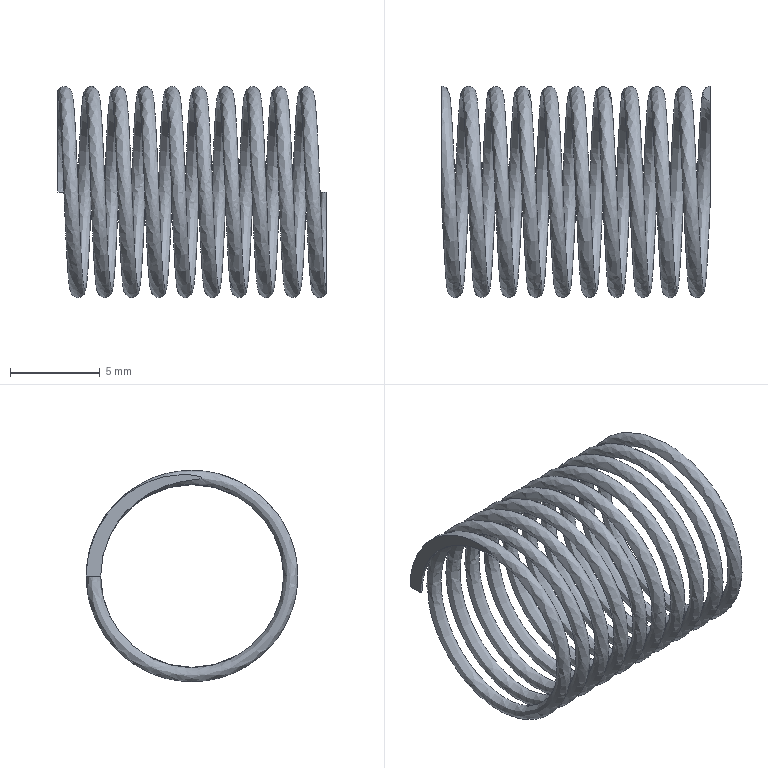Part | NX | features BREP 1, DATUM_CSYS 1 | 1 solid | 5 faces | box 15 x 11.8 x 11.8 mm | volume 171.601 mm3 | plane 4 | spline 1
STEP:
#1=CARTESIAN_POINT('',(76.,5.1,8.));
#2=VERTEX_POINT('',#1);
#3=CARTESIAN_POINT('',(76.,5.9,8.));
#4=VERTEX_POINT('',#3);
#5=CARTESIAN_POINT('',(76.,5.5,8.));
#6=DIRECTION('',(0.,0.,-1.));
#7=DIRECTION('',(0.,-1.,0.));
#8=AXIS2_PLACEMENT_3D('',#5,#6,#7);
#9=CIRCLE('',#8,0.4);
#10=EDGE_CURVE('',#2,#4,#9,.T.);
#11=ORIENTED_EDGE('',*,*,#10,.F.);
#12=CARTESIAN_POINT('',(76.,5.9,8.));
#13=DIRECTION('',(0.,-1.,0.));
#14=VECTOR('',#13,1000.);
#15=LINE('',#12,#14);
#16=EDGE_CURVE('',#4,#2,#15,.T.);
#17=ORIENTED_EDGE('',*,*,#16,.F.);
#18=EDGE_LOOP('',(#11,#17));
#19=FACE_BOUND('',#18,.T.);
#20=CARTESIAN_POINT('',(75.8,5.5,8.));
#21=DIRECTION('',(0.,0.,1.));
#22=DIRECTION('',(0.,-1.,0.));
#23=AXIS2_PLACEMENT_3D('',#20,#21,#22);
#24=PLANE('',#23);
#25=ADVANCED_FACE('',(#19),#24,.T.);
#26=CARTESIAN_POINT('',(76.,-0.5373,2.526));
#27=VERTEX_POINT('',#26);
#28=CARTESIAN_POINT('',(61.4,5.5,8.));
#29=VERTEX_POINT('',#28);
#30=CARTESIAN_POINT('',(76.,-0.5373,2.526));
#31=CARTESIAN_POINT('',(75.843,-3.895,2.856));
#32=CARTESIAN_POINT('',(75.761,-5.5,5.447));
#33=CARTESIAN_POINT('',(75.65,-5.5,8.));
#34=CARTESIAN_POINT('',(75.173,-5.5,19.));
#35=CARTESIAN_POINT('',(75.377,5.5,19.));
#36=CARTESIAN_POINT('',(74.9,5.5,8.));
#37=CARTESIAN_POINT('',(74.423,5.5,-3.));
#38=CARTESIAN_POINT('',(74.627,-5.5,-3.));
#39=CARTESIAN_POINT('',(74.15,-5.5,8.));
#40=CARTESIAN_POINT('',(73.673,-5.5,19.));
#41=CARTESIAN_POINT('',(73.877,5.5,19.));
#42=CARTESIAN_POINT('',(73.4,5.5,8.));
#43=CARTESIAN_POINT('',(72.923,5.5,-3.));
#44=CARTESIAN_POINT('',(73.127,-5.5,-3.));
#45=CARTESIAN_POINT('',(72.65,-5.5,8.));
#46=CARTESIAN_POINT('',(72.173,-5.5,19.));
#47=CARTESIAN_POINT('',(72.377,5.5,19.));
#48=CARTESIAN_POINT('',(71.9,5.5,8.));
#49=CARTESIAN_POINT('',(71.423,5.5,-3.));
#50=CARTESIAN_POINT('',(71.627,-5.5,-3.));
#51=CARTESIAN_POINT('',(71.15,-5.5,8.));
#52=CARTESIAN_POINT('',(70.673,-5.5,19.));
#53=CARTESIAN_POINT('',(70.877,5.5,19.));
#54=CARTESIAN_POINT('',(70.4,5.5,8.));
#55=CARTESIAN_POINT('',(69.923,5.5,-3.));
#56=CARTESIAN_POINT('',(70.127,-5.5,-3.));
#57=CARTESIAN_POINT('',(69.65,-5.5,8.));
#58=CARTESIAN_POINT('',(69.173,-5.5,19.));
#59=CARTESIAN_POINT('',(69.377,5.5,19.));
#60=CARTESIAN_POINT('',(68.9,5.5,8.));
#61=CARTESIAN_POINT('',(68.423,5.5,-3.));
#62=CARTESIAN_POINT('',(68.627,-5.5,-3.));
#63=CARTESIAN_POINT('',(68.15,-5.5,8.));
#64=CARTESIAN_POINT('',(67.673,-5.5,19.));
#65=CARTESIAN_POINT('',(67.877,5.5,19.));
#66=CARTESIAN_POINT('',(67.4,5.5,8.));
#67=CARTESIAN_POINT('',(66.923,5.5,-3.));
#68=CARTESIAN_POINT('',(67.127,-5.5,-3.));
#69=CARTESIAN_POINT('',(66.65,-5.5,8.));
#70=CARTESIAN_POINT('',(66.173,-5.5,19.));
#71=CARTESIAN_POINT('',(66.377,5.5,19.));
#72=CARTESIAN_POINT('',(65.9,5.5,8.));
#73=CARTESIAN_POINT('',(65.423,5.5,-3.));
#74=CARTESIAN_POINT('',(65.627,-5.5,-3.));
#75=CARTESIAN_POINT('',(65.15,-5.5,8.));
#76=CARTESIAN_POINT('',(64.673,-5.5,19.));
#77=CARTESIAN_POINT('',(64.877,5.5,19.));
#78=CARTESIAN_POINT('',(64.4,5.5,8.));
#79=CARTESIAN_POINT('',(63.923,5.5,-3.));
#80=CARTESIAN_POINT('',(64.127,-5.5,-3.));
#81=CARTESIAN_POINT('',(63.65,-5.5,8.));
#82=CARTESIAN_POINT('',(63.173,-5.5,19.));
#83=CARTESIAN_POINT('',(63.377,5.5,19.));
#84=CARTESIAN_POINT('',(62.9,5.5,8.));
#85=CARTESIAN_POINT('',(62.423,5.5,-3.));
#86=CARTESIAN_POINT('',(62.627,-5.5,-3.));
#87=CARTESIAN_POINT('',(62.15,-5.5,8.));
#88=CARTESIAN_POINT('',(61.673,-5.5,19.));
#89=CARTESIAN_POINT('',(61.877,5.5,19.));
#90=CARTESIAN_POINT('',(61.4,5.5,8.));
#91=(BOUNDED_CURVE()B_SPLINE_CURVE(3,(#30,#31,#32,#33,#34,#35,#36,#37,#38,#39,#40,#41,#42,#43,#44,#45,#46,#47,#48,#49,#50,#51,#52,#53,#54,#55,#56,#57,#58,#59,#60,#61,#62,#63,#64,#65,#66,#67,#68,#69,#70,#71,#72,#73,#74,#75,#76,#77,#78,#79,#80,#81,#82,#83,#84,#85,#86,#87,#88,#89,#90),.UNSPECIFIED.,.F.,.F.)B_SPLINE_CURVE_WITH_KNOTS((4,3,3,3,3,3,3,3,3,3,3,3,3,3,3,3,3,3,3,3,4),(0.,0.02442,0.07576,0.1271,0.1785,0.2298,0.2811,0.3325,0.3838,0.4352,0.4865,0.5379,0.5892,0.6406,0.6919,0.7433,0.7946,0.846,0.8973,0.9487,1.),.PIECEWISE_BEZIER_KNOTS.)CURVE()GEOMETRIC_REPRESENTATION_ITEM()RATIONAL_B_SPLINE_CURVE((0.5012,0.5167,0.683,1.,0.3333,0.3333,1.,0.3333,0.3333,1.,0.3333,0.3333,1.,0.3333,0.3333,1.,0.3333,0.3333,1.,0.3333,0.3333,1.,0.3333,0.3333,1.,0.3333,0.3333,1.,0.3333,0.3333,1.,0.3333,0.3333,1.,0.3333,0.3333,1.,0.3333,0.3333,1.,0.3333,0.3333,1.,0.3333,0.3333,1.,0.3333,0.3333,1.,0.3333,0.3333,1.,0.3333,0.3333,1.,0.3333,0.3333,1.,0.3333,0.3333,1.))REPRESENTATION_ITEM(''));
#92=EDGE_CURVE('',#27,#29,#91,.T.);
#93=ORIENTED_EDGE('',*,*,#92,.F.);
#94=CARTESIAN_POINT('',(76.,5.1,8.));
#95=CARTESIAN_POINT('',(76.,5.1,7.271));
#96=CARTESIAN_POINT('',(76.,4.87,6.189));
#97=CARTESIAN_POINT('',(76.,4.149,4.925));
#98=CARTESIAN_POINT('',(76.,3.427,4.106));
#99=CARTESIAN_POINT('',(76.,2.563,3.453));
#100=CARTESIAN_POINT('',(76.,1.74,3.054));
#101=CARTESIAN_POINT('',(76.,1.056,2.834));
#102=CARTESIAN_POINT('',(76.,0.5256,2.714));
#103=CARTESIAN_POINT('',(76.,0.08176,2.645));
#104=CARTESIAN_POINT('',(76.,-0.2455,2.613));
#105=CARTESIAN_POINT('',(76.,-0.4071,2.578));
#106=CARTESIAN_POINT('',(76.,-0.5328,2.572));
#107=CARTESIAN_POINT('',(76.,-0.5373,2.526));
#108=B_SPLINE_CURVE_WITH_KNOTS('',3,(#94,#95,#96,#97,#98,#99,#100,#101,#102,#103,#104,#105,#106,#107),.UNSPECIFIED.,.F.,.F.,(4,1,1,1,1,1,1,1,1,1,1,4),(0.,0.002182,0.003272,0.004363,0.005454,0.006545,0.00709,0.007636,0.008181,0.008454,0.00859,0.008726),.UNSPECIFIED.);
#109=EDGE_CURVE('',#2,#27,#108,.T.);
#110=ORIENTED_EDGE('',*,*,#109,.F.);
#111=ORIENTED_EDGE('',*,*,#10,.T.);
#112=CARTESIAN_POINT('',(76.,-0.5373,2.526));
#113=CARTESIAN_POINT('',(76.,-0.5425,2.474));
#114=CARTESIAN_POINT('',(76.,-0.3977,2.446));
#115=CARTESIAN_POINT('',(76.,-0.2237,2.388));
#116=CARTESIAN_POINT('',(76.,0.04228,2.353));
#117=CARTESIAN_POINT('',(76.,0.3421,2.331));
#118=CARTESIAN_POINT('',(76.,0.7489,2.333));
#119=CARTESIAN_POINT('',(76.,1.259,2.386));
#120=CARTESIAN_POINT('',(76.,2.047,2.563));
#121=CARTESIAN_POINT('',(76.,2.993,2.956));
#122=CARTESIAN_POINT('',(76.,3.989,3.658));
#123=CARTESIAN_POINT('',(76.,4.817,4.562));
#124=CARTESIAN_POINT('',(76.,5.639,5.973));
#125=CARTESIAN_POINT('',(76.,5.9,7.182));
#126=CARTESIAN_POINT('',(76.,5.9,8.));
#127=B_SPLINE_CURVE_WITH_KNOTS('',3,(#112,#113,#114,#115,#116,#117,#118,#119,#120,#121,#122,#123,#124,#125,#126),.UNSPECIFIED.,.F.,.F.,(4,1,1,1,1,1,1,1,1,1,1,1,4),(0.,0.0001559,0.0003119,0.0006238,0.0009356,0.001248,0.001871,0.002495,0.003743,0.00499,0.006238,0.007485,0.00998),.UNSPECIFIED.);
#128=EDGE_CURVE('',#27,#4,#127,.T.);
#129=ORIENTED_EDGE('',*,*,#128,.F.);
#130=ORIENTED_EDGE('',*,*,#92,.T.);
#131=CARTESIAN_POINT('',(61.,5.9,8.));
#132=VERTEX_POINT('',#131);
#133=CARTESIAN_POINT('',(61.,5.9,8.));
#134=CARTESIAN_POINT('',(61.4,5.9,8.));
#135=CARTESIAN_POINT('',(61.4,5.5,8.));
#136=(BOUNDED_CURVE()B_SPLINE_CURVE(2,(#133,#134,#135),.UNSPECIFIED.,.F.,.F.)B_SPLINE_CURVE_WITH_KNOTS((3,3),(0.,1.),.PIECEWISE_BEZIER_KNOTS.)CURVE()GEOMETRIC_REPRESENTATION_ITEM()RATIONAL_B_SPLINE_CURVE((0.8038,0.634,1.))REPRESENTATION_ITEM(''));
#137=EDGE_CURVE('',#132,#29,#136,.T.);
#138=ORIENTED_EDGE('',*,*,#137,.F.);
#139=CARTESIAN_POINT('',(61.,5.1,8.));
#140=VERTEX_POINT('',#139);
#141=CARTESIAN_POINT('',(61.,5.1,8.));
#142=CARTESIAN_POINT('',(61.,5.1,8.783));
#143=CARTESIAN_POINT('',(61.,4.747,10.331));
#144=CARTESIAN_POINT('',(61.,3.515,11.895));
#145=CARTESIAN_POINT('',(61.,2.218,12.748));
#146=CARTESIAN_POINT('',(61.,1.309,13.105));
#147=CARTESIAN_POINT('',(61.,0.5535,13.282));
#148=CARTESIAN_POINT('',(61.,0.07717,13.354));
#149=CARTESIAN_POINT('',(61.,-0.2742,13.393));
#150=CARTESIAN_POINT('',(61.,-0.4254,13.421));
#151=CARTESIAN_POINT('',(61.,-0.5471,13.447));
#152=CARTESIAN_POINT('',(61.,-0.4994,13.543));
#153=CARTESIAN_POINT('',(61.,-0.3702,13.564));
#154=CARTESIAN_POINT('',(61.,-0.1891,13.617));
#155=CARTESIAN_POINT('',(61.,0.145,13.66));
#156=CARTESIAN_POINT('',(61.,0.6237,13.677));
#157=CARTESIAN_POINT('',(61.,1.379,13.606));
#158=CARTESIAN_POINT('',(61.,2.307,13.358));
#159=CARTESIAN_POINT('',(61.,3.323,12.839));
#160=CARTESIAN_POINT('',(61.,4.517,11.882));
#161=CARTESIAN_POINT('',(61.,5.594,10.279));
#162=CARTESIAN_POINT('',(61.,5.9,8.766));
#163=CARTESIAN_POINT('',(61.,5.9,8.));
#164=B_SPLINE_CURVE_WITH_KNOTS('',3,(#141,#142,#143,#144,#145,#146,#147,#148,#149,#150,#151,#152,#153,#154,#155,#156,#157,#158,#159,#160,#161,#162,#163),.UNSPECIFIED.,.F.,.F.,(4,1,1,1,1,1,1,1,1,1,1,1,1,1,1,1,1,1,1,1,4),(0.,0.002341,0.004682,0.005852,0.007022,0.007608,0.008193,0.008485,0.008632,0.008705,0.008778,0.008924,0.00907,0.009363,0.009948,0.01053,0.0117,0.01287,0.01404,0.01639,0.01873),.UNSPECIFIED.);
#165=EDGE_CURVE('',#140,#132,#164,.T.);
#166=ORIENTED_EDGE('',*,*,#165,.F.);
#167=CARTESIAN_POINT('',(61.4,5.5,8.));
#168=CARTESIAN_POINT('',(61.4,5.1,8.));
#169=CARTESIAN_POINT('',(61.,5.1,8.));
#170=(BOUNDED_CURVE()B_SPLINE_CURVE(2,(#167,#168,#169),.UNSPECIFIED.,.F.,.F.)B_SPLINE_CURVE_WITH_KNOTS((3,3),(0.,1.),.PIECEWISE_BEZIER_KNOTS.)CURVE()GEOMETRIC_REPRESENTATION_ITEM()RATIONAL_B_SPLINE_CURVE((1.,0.634,0.8038))REPRESENTATION_ITEM(''));
#171=EDGE_CURVE('',#29,#140,#170,.T.);
#172=ORIENTED_EDGE('',*,*,#171,.F.);
#173=EDGE_LOOP('',(#93,#110,#111,#129,#130,#138,#166,#172));
#174=FACE_BOUND('',#173,.T.);
#175=CARTESIAN_POINT('',(76.4,5.5,8.));
#176=CARTESIAN_POINT('',(75.923,5.5,-3.));
#177=CARTESIAN_POINT('',(76.127,-5.5,-3.));
#178=CARTESIAN_POINT('',(75.65,-5.5,8.));
#179=CARTESIAN_POINT('',(75.173,-5.5,19.));
#180=CARTESIAN_POINT('',(75.377,5.5,19.));
#181=CARTESIAN_POINT('',(74.9,5.5,8.));
#182=CARTESIAN_POINT('',(74.423,5.5,-3.));
#183=CARTESIAN_POINT('',(74.627,-5.5,-3.));
#184=CARTESIAN_POINT('',(74.15,-5.5,8.));
#185=CARTESIAN_POINT('',(73.673,-5.5,19.));
#186=CARTESIAN_POINT('',(73.877,5.5,19.));
#187=CARTESIAN_POINT('',(73.4,5.5,8.));
#188=CARTESIAN_POINT('',(72.923,5.5,-3.));
#189=CARTESIAN_POINT('',(73.127,-5.5,-3.));
#190=CARTESIAN_POINT('',(72.65,-5.5,8.));
#191=CARTESIAN_POINT('',(72.173,-5.5,19.));
#192=CARTESIAN_POINT('',(72.377,5.5,19.));
#193=CARTESIAN_POINT('',(71.9,5.5,8.));
#194=CARTESIAN_POINT('',(71.423,5.5,-3.));
#195=CARTESIAN_POINT('',(71.627,-5.5,-3.));
#196=CARTESIAN_POINT('',(71.15,-5.5,8.));
#197=CARTESIAN_POINT('',(70.673,-5.5,19.));
#198=CARTESIAN_POINT('',(70.877,5.5,19.));
#199=CARTESIAN_POINT('',(70.4,5.5,8.));
#200=CARTESIAN_POINT('',(69.923,5.5,-3.));
#201=CARTESIAN_POINT('',(70.127,-5.5,-3.));
#202=CARTESIAN_POINT('',(69.65,-5.5,8.));
#203=CARTESIAN_POINT('',(69.173,-5.5,19.));
#204=CARTESIAN_POINT('',(69.377,5.5,19.));
#205=CARTESIAN_POINT('',(68.9,5.5,8.));
#206=CARTESIAN_POINT('',(68.423,5.5,-3.));
#207=CARTESIAN_POINT('',(68.627,-5.5,-3.));
#208=CARTESIAN_POINT('',(68.15,-5.5,8.));
#209=CARTESIAN_POINT('',(67.673,-5.5,19.));
#210=CARTESIAN_POINT('',(67.877,5.5,19.));
#211=CARTESIAN_POINT('',(67.4,5.5,8.));
#212=CARTESIAN_POINT('',(66.923,5.5,-3.));
#213=CARTESIAN_POINT('',(67.127,-5.5,-3.));
#214=CARTESIAN_POINT('',(66.65,-5.5,8.));
#215=CARTESIAN_POINT('',(66.173,-5.5,19.));
#216=CARTESIAN_POINT('',(66.377,5.5,19.));
#217=CARTESIAN_POINT('',(65.9,5.5,8.));
#218=CARTESIAN_POINT('',(65.423,5.5,-3.));
#219=CARTESIAN_POINT('',(65.627,-5.5,-3.));
#220=CARTESIAN_POINT('',(65.15,-5.5,8.));
#221=CARTESIAN_POINT('',(64.673,-5.5,19.));
#222=CARTESIAN_POINT('',(64.877,5.5,19.));
#223=CARTESIAN_POINT('',(64.4,5.5,8.));
#224=CARTESIAN_POINT('',(63.923,5.5,-3.));
#225=CARTESIAN_POINT('',(64.127,-5.5,-3.));
#226=CARTESIAN_POINT('',(63.65,-5.5,8.));
#227=CARTESIAN_POINT('',(63.173,-5.5,19.));
#228=CARTESIAN_POINT('',(63.377,5.5,19.));
#229=CARTESIAN_POINT('',(62.9,5.5,8.));
#230=CARTESIAN_POINT('',(62.423,5.5,-3.));
#231=CARTESIAN_POINT('',(62.627,-5.5,-3.));
#232=CARTESIAN_POINT('',(62.15,-5.5,8.));
#233=CARTESIAN_POINT('',(61.673,-5.5,19.));
#234=CARTESIAN_POINT('',(61.877,5.5,19.));
#235=CARTESIAN_POINT('',(61.4,5.5,8.));
#236=CARTESIAN_POINT('',(76.4,4.807,8.));
#237=CARTESIAN_POINT('',(75.923,4.807,-1.614));
#238=CARTESIAN_POINT('',(76.127,-4.807,-1.614));
#239=CARTESIAN_POINT('',(75.65,-4.807,8.));
#240=CARTESIAN_POINT('',(75.173,-4.807,17.614));
#241=CARTESIAN_POINT('',(75.377,4.807,17.614));
#242=CARTESIAN_POINT('',(74.9,4.807,8.));
#243=CARTESIAN_POINT('',(74.423,4.807,-1.614));
#244=CARTESIAN_POINT('',(74.627,-4.807,-1.614));
#245=CARTESIAN_POINT('',(74.15,-4.807,8.));
#246=CARTESIAN_POINT('',(73.673,-4.807,17.614));
#247=CARTESIAN_POINT('',(73.877,4.807,17.614));
#248=CARTESIAN_POINT('',(73.4,4.807,8.));
#249=CARTESIAN_POINT('',(72.923,4.807,-1.614));
#250=CARTESIAN_POINT('',(73.127,-4.807,-1.614));
#251=CARTESIAN_POINT('',(72.65,-4.807,8.));
#252=CARTESIAN_POINT('',(72.173,-4.807,17.614));
#253=CARTESIAN_POINT('',(72.377,4.807,17.614));
#254=CARTESIAN_POINT('',(71.9,4.807,8.));
#255=CARTESIAN_POINT('',(71.423,4.807,-1.614));
#256=CARTESIAN_POINT('',(71.627,-4.807,-1.614));
#257=CARTESIAN_POINT('',(71.15,-4.807,8.));
#258=CARTESIAN_POINT('',(70.673,-4.807,17.614));
#259=CARTESIAN_POINT('',(70.877,4.807,17.614));
#260=CARTESIAN_POINT('',(70.4,4.807,8.));
#261=CARTESIAN_POINT('',(69.923,4.807,-1.614));
#262=CARTESIAN_POINT('',(70.127,-4.807,-1.614));
#263=CARTESIAN_POINT('',(69.65,-4.807,8.));
#264=CARTESIAN_POINT('',(69.173,-4.807,17.614));
#265=CARTESIAN_POINT('',(69.377,4.807,17.614));
#266=CARTESIAN_POINT('',(68.9,4.807,8.));
#267=CARTESIAN_POINT('',(68.423,4.807,-1.614));
#268=CARTESIAN_POINT('',(68.627,-4.807,-1.614));
#269=CARTESIAN_POINT('',(68.15,-4.807,8.));
#270=CARTESIAN_POINT('',(67.673,-4.807,17.614));
#271=CARTESIAN_POINT('',(67.877,4.807,17.614));
#272=CARTESIAN_POINT('',(67.4,4.807,8.));
#273=CARTESIAN_POINT('',(66.923,4.807,-1.614));
#274=CARTESIAN_POINT('',(67.127,-4.807,-1.614));
#275=CARTESIAN_POINT('',(66.65,-4.807,8.));
#276=CARTESIAN_POINT('',(66.173,-4.807,17.614));
#277=CARTESIAN_POINT('',(66.377,4.807,17.614));
#278=CARTESIAN_POINT('',(65.9,4.807,8.));
#279=CARTESIAN_POINT('',(65.423,4.807,-1.614));
#280=CARTESIAN_POINT('',(65.627,-4.807,-1.614));
#281=CARTESIAN_POINT('',(65.15,-4.807,8.));
#282=CARTESIAN_POINT('',(64.673,-4.807,17.614));
#283=CARTESIAN_POINT('',(64.877,4.807,17.614));
#284=CARTESIAN_POINT('',(64.4,4.807,8.));
#285=CARTESIAN_POINT('',(63.923,4.807,-1.614));
#286=CARTESIAN_POINT('',(64.127,-4.807,-1.614));
#287=CARTESIAN_POINT('',(63.65,-4.807,8.));
#288=CARTESIAN_POINT('',(63.173,-4.807,17.614));
#289=CARTESIAN_POINT('',(63.377,4.807,17.614));
#290=CARTESIAN_POINT('',(62.9,4.807,8.));
#291=CARTESIAN_POINT('',(62.423,4.807,-1.614));
#292=CARTESIAN_POINT('',(62.627,-4.807,-1.614));
#293=CARTESIAN_POINT('',(62.15,-4.807,8.));
#294=CARTESIAN_POINT('',(61.673,-4.807,17.614));
#295=CARTESIAN_POINT('',(61.877,4.807,17.614));
#296=CARTESIAN_POINT('',(61.4,4.807,8.));
#297=CARTESIAN_POINT('',(75.8,5.154,8.));
#298=CARTESIAN_POINT('',(75.323,5.154,-2.307));
#299=CARTESIAN_POINT('',(75.527,-5.154,-2.307));
#300=CARTESIAN_POINT('',(75.05,-5.154,8.));
#301=CARTESIAN_POINT('',(74.573,-5.154,18.307));
#302=CARTESIAN_POINT('',(74.777,5.154,18.307));
#303=CARTESIAN_POINT('',(74.3,5.154,8.));
#304=CARTESIAN_POINT('',(73.823,5.154,-2.307));
#305=CARTESIAN_POINT('',(74.027,-5.154,-2.307));
#306=CARTESIAN_POINT('',(73.55,-5.154,8.));
#307=CARTESIAN_POINT('',(73.073,-5.154,18.307));
#308=CARTESIAN_POINT('',(73.277,5.154,18.307));
#309=CARTESIAN_POINT('',(72.8,5.154,8.));
#310=CARTESIAN_POINT('',(72.323,5.154,-2.307));
#311=CARTESIAN_POINT('',(72.527,-5.154,-2.307));
#312=CARTESIAN_POINT('',(72.05,-5.154,8.));
#313=CARTESIAN_POINT('',(71.573,-5.154,18.307));
#314=CARTESIAN_POINT('',(71.777,5.154,18.307));
#315=CARTESIAN_POINT('',(71.3,5.154,8.));
#316=CARTESIAN_POINT('',(70.823,5.154,-2.307));
#317=CARTESIAN_POINT('',(71.027,-5.154,-2.307));
#318=CARTESIAN_POINT('',(70.55,-5.154,8.));
#319=CARTESIAN_POINT('',(70.073,-5.154,18.307));
#320=CARTESIAN_POINT('',(70.277,5.154,18.307));
#321=CARTESIAN_POINT('',(69.8,5.154,8.));
#322=CARTESIAN_POINT('',(69.323,5.154,-2.307));
#323=CARTESIAN_POINT('',(69.527,-5.154,-2.307));
#324=CARTESIAN_POINT('',(69.05,-5.154,8.));
#325=CARTESIAN_POINT('',(68.573,-5.154,18.307));
#326=CARTESIAN_POINT('',(68.777,5.154,18.307));
#327=CARTESIAN_POINT('',(68.3,5.154,8.));
#328=CARTESIAN_POINT('',(67.823,5.154,-2.307));
#329=CARTESIAN_POINT('',(68.027,-5.154,-2.307));
#330=CARTESIAN_POINT('',(67.55,-5.154,8.));
#331=CARTESIAN_POINT('',(67.073,-5.154,18.307));
#332=CARTESIAN_POINT('',(67.277,5.154,18.307));
#333=CARTESIAN_POINT('',(66.8,5.154,8.));
#334=CARTESIAN_POINT('',(66.323,5.154,-2.307));
#335=CARTESIAN_POINT('',(66.527,-5.154,-2.307));
#336=CARTESIAN_POINT('',(66.05,-5.154,8.));
#337=CARTESIAN_POINT('',(65.573,-5.154,18.307));
#338=CARTESIAN_POINT('',(65.777,5.154,18.307));
#339=CARTESIAN_POINT('',(65.3,5.154,8.));
#340=CARTESIAN_POINT('',(64.823,5.154,-2.307));
#341=CARTESIAN_POINT('',(65.027,-5.154,-2.307));
#342=CARTESIAN_POINT('',(64.55,-5.154,8.));
#343=CARTESIAN_POINT('',(64.073,-5.154,18.307));
#344=CARTESIAN_POINT('',(64.277,5.154,18.307));
#345=CARTESIAN_POINT('',(63.8,5.154,8.));
#346=CARTESIAN_POINT('',(63.323,5.154,-2.307));
#347=CARTESIAN_POINT('',(63.527,-5.154,-2.307));
#348=CARTESIAN_POINT('',(63.05,-5.154,8.));
#349=CARTESIAN_POINT('',(62.573,-5.154,18.307));
#350=CARTESIAN_POINT('',(62.777,5.154,18.307));
#351=CARTESIAN_POINT('',(62.3,5.154,8.));
#352=CARTESIAN_POINT('',(61.823,5.154,-2.307));
#353=CARTESIAN_POINT('',(62.027,-5.154,-2.307));
#354=CARTESIAN_POINT('',(61.55,-5.154,8.));
#355=CARTESIAN_POINT('',(61.073,-5.154,18.307));
#356=CARTESIAN_POINT('',(61.277,5.154,18.307));
#357=CARTESIAN_POINT('',(60.8,5.154,8.));
#358=CARTESIAN_POINT('',(75.2,5.5,8.));
#359=CARTESIAN_POINT('',(74.723,5.5,-3.));
#360=CARTESIAN_POINT('',(74.927,-5.5,-3.));
#361=CARTESIAN_POINT('',(74.45,-5.5,8.));
#362=CARTESIAN_POINT('',(73.973,-5.5,19.));
#363=CARTESIAN_POINT('',(74.177,5.5,19.));
#364=CARTESIAN_POINT('',(73.7,5.5,8.));
#365=CARTESIAN_POINT('',(73.223,5.5,-3.));
#366=CARTESIAN_POINT('',(73.427,-5.5,-3.));
#367=CARTESIAN_POINT('',(72.95,-5.5,8.));
#368=CARTESIAN_POINT('',(72.473,-5.5,19.));
#369=CARTESIAN_POINT('',(72.677,5.5,19.));
#370=CARTESIAN_POINT('',(72.2,5.5,8.));
#371=CARTESIAN_POINT('',(71.723,5.5,-3.));
#372=CARTESIAN_POINT('',(71.927,-5.5,-3.));
#373=CARTESIAN_POINT('',(71.45,-5.5,8.));
#374=CARTESIAN_POINT('',(70.973,-5.5,19.));
#375=CARTESIAN_POINT('',(71.177,5.5,19.));
#376=CARTESIAN_POINT('',(70.7,5.5,8.));
#377=CARTESIAN_POINT('',(70.223,5.5,-3.));
#378=CARTESIAN_POINT('',(70.427,-5.5,-3.));
#379=CARTESIAN_POINT('',(69.95,-5.5,8.));
#380=CARTESIAN_POINT('',(69.473,-5.5,19.));
#381=CARTESIAN_POINT('',(69.677,5.5,19.));
#382=CARTESIAN_POINT('',(69.2,5.5,8.));
#383=CARTESIAN_POINT('',(68.723,5.5,-3.));
#384=CARTESIAN_POINT('',(68.927,-5.5,-3.));
#385=CARTESIAN_POINT('',(68.45,-5.5,8.));
#386=CARTESIAN_POINT('',(67.973,-5.5,19.));
#387=CARTESIAN_POINT('',(68.177,5.5,19.));
#388=CARTESIAN_POINT('',(67.7,5.5,8.));
#389=CARTESIAN_POINT('',(67.223,5.5,-3.));
#390=CARTESIAN_POINT('',(67.427,-5.5,-3.));
#391=CARTESIAN_POINT('',(66.95,-5.5,8.));
#392=CARTESIAN_POINT('',(66.473,-5.5,19.));
#393=CARTESIAN_POINT('',(66.677,5.5,19.));
#394=CARTESIAN_POINT('',(66.2,5.5,8.));
#395=CARTESIAN_POINT('',(65.723,5.5,-3.));
#396=CARTESIAN_POINT('',(65.927,-5.5,-3.));
#397=CARTESIAN_POINT('',(65.45,-5.5,8.));
#398=CARTESIAN_POINT('',(64.973,-5.5,19.));
#399=CARTESIAN_POINT('',(65.177,5.5,19.));
#400=CARTESIAN_POINT('',(64.7,5.5,8.));
#401=CARTESIAN_POINT('',(64.223,5.5,-3.));
#402=CARTESIAN_POINT('',(64.427,-5.5,-3.));
#403=CARTESIAN_POINT('',(63.95,-5.5,8.));
#404=CARTESIAN_POINT('',(63.473,-5.5,19.));
#405=CARTESIAN_POINT('',(63.677,5.5,19.));
#406=CARTESIAN_POINT('',(63.2,5.5,8.));
#407=CARTESIAN_POINT('',(62.723,5.5,-3.));
#408=CARTESIAN_POINT('',(62.927,-5.5,-3.));
#409=CARTESIAN_POINT('',(62.45,-5.5,8.));
#410=CARTESIAN_POINT('',(61.973,-5.5,19.));
#411=CARTESIAN_POINT('',(62.177,5.5,19.));
#412=CARTESIAN_POINT('',(61.7,5.5,8.));
#413=CARTESIAN_POINT('',(61.223,5.5,-3.));
#414=CARTESIAN_POINT('',(61.427,-5.5,-3.));
#415=CARTESIAN_POINT('',(60.95,-5.5,8.));
#416=CARTESIAN_POINT('',(60.473,-5.5,19.));
#417=CARTESIAN_POINT('',(60.677,5.5,19.));
#418=CARTESIAN_POINT('',(60.2,5.5,8.));
#419=CARTESIAN_POINT('',(75.8,5.846,8.));
#420=CARTESIAN_POINT('',(75.323,5.846,-3.693));
#421=CARTESIAN_POINT('',(75.527,-5.846,-3.693));
#422=CARTESIAN_POINT('',(75.05,-5.846,8.));
#423=CARTESIAN_POINT('',(74.573,-5.846,19.693));
#424=CARTESIAN_POINT('',(74.777,5.846,19.693));
#425=CARTESIAN_POINT('',(74.3,5.846,8.));
#426=CARTESIAN_POINT('',(73.823,5.846,-3.693));
#427=CARTESIAN_POINT('',(74.027,-5.846,-3.693));
#428=CARTESIAN_POINT('',(73.55,-5.846,8.));
#429=CARTESIAN_POINT('',(73.073,-5.846,19.693));
#430=CARTESIAN_POINT('',(73.277,5.846,19.693));
#431=CARTESIAN_POINT('',(72.8,5.846,8.));
#432=CARTESIAN_POINT('',(72.323,5.846,-3.693));
#433=CARTESIAN_POINT('',(72.527,-5.846,-3.693));
#434=CARTESIAN_POINT('',(72.05,-5.846,8.));
#435=CARTESIAN_POINT('',(71.573,-5.846,19.693));
#436=CARTESIAN_POINT('',(71.777,5.846,19.693));
#437=CARTESIAN_POINT('',(71.3,5.846,8.));
#438=CARTESIAN_POINT('',(70.823,5.846,-3.693));
#439=CARTESIAN_POINT('',(71.027,-5.846,-3.693));
#440=CARTESIAN_POINT('',(70.55,-5.846,8.));
#441=CARTESIAN_POINT('',(70.073,-5.846,19.693));
#442=CARTESIAN_POINT('',(70.277,5.846,19.693));
#443=CARTESIAN_POINT('',(69.8,5.846,8.));
#444=CARTESIAN_POINT('',(69.323,5.846,-3.693));
#445=CARTESIAN_POINT('',(69.527,-5.846,-3.693));
#446=CARTESIAN_POINT('',(69.05,-5.846,8.));
#447=CARTESIAN_POINT('',(68.573,-5.846,19.693));
#448=CARTESIAN_POINT('',(68.777,5.846,19.693));
#449=CARTESIAN_POINT('',(68.3,5.846,8.));
#450=CARTESIAN_POINT('',(67.823,5.846,-3.693));
#451=CARTESIAN_POINT('',(68.027,-5.846,-3.693));
#452=CARTESIAN_POINT('',(67.55,-5.846,8.));
#453=CARTESIAN_POINT('',(67.073,-5.846,19.693));
#454=CARTESIAN_POINT('',(67.277,5.846,19.693));
#455=CARTESIAN_POINT('',(66.8,5.846,8.));
#456=CARTESIAN_POINT('',(66.323,5.846,-3.693));
#457=CARTESIAN_POINT('',(66.527,-5.846,-3.693));
#458=CARTESIAN_POINT('',(66.05,-5.846,8.));
#459=CARTESIAN_POINT('',(65.573,-5.846,19.693));
#460=CARTESIAN_POINT('',(65.777,5.846,19.693));
#461=CARTESIAN_POINT('',(65.3,5.846,8.));
#462=CARTESIAN_POINT('',(64.823,5.846,-3.693));
#463=CARTESIAN_POINT('',(65.027,-5.846,-3.693));
#464=CARTESIAN_POINT('',(64.55,-5.846,8.));
#465=CARTESIAN_POINT('',(64.073,-5.846,19.693));
#466=CARTESIAN_POINT('',(64.277,5.846,19.693));
#467=CARTESIAN_POINT('',(63.8,5.846,8.));
#468=CARTESIAN_POINT('',(63.323,5.846,-3.693));
#469=CARTESIAN_POINT('',(63.527,-5.846,-3.693));
#470=CARTESIAN_POINT('',(63.05,-5.846,8.));
#471=CARTESIAN_POINT('',(62.573,-5.846,19.693));
#472=CARTESIAN_POINT('',(62.777,5.846,19.693));
#473=CARTESIAN_POINT('',(62.3,5.846,8.));
#474=CARTESIAN_POINT('',(61.823,5.846,-3.693));
#475=CARTESIAN_POINT('',(62.027,-5.846,-3.693));
#476=CARTESIAN_POINT('',(61.55,-5.846,8.));
#477=CARTESIAN_POINT('',(61.073,-5.846,19.693));
#478=CARTESIAN_POINT('',(61.277,5.846,19.693));
#479=CARTESIAN_POINT('',(60.8,5.846,8.));
#480=CARTESIAN_POINT('',(76.4,6.193,8.));
#481=CARTESIAN_POINT('',(75.923,6.193,-4.386));
#482=CARTESIAN_POINT('',(76.127,-6.193,-4.386));
#483=CARTESIAN_POINT('',(75.65,-6.193,8.));
#484=CARTESIAN_POINT('',(75.173,-6.193,20.386));
#485=CARTESIAN_POINT('',(75.377,6.193,20.386));
#486=CARTESIAN_POINT('',(74.9,6.193,8.));
#487=CARTESIAN_POINT('',(74.423,6.193,-4.386));
#488=CARTESIAN_POINT('',(74.627,-6.193,-4.386));
#489=CARTESIAN_POINT('',(74.15,-6.193,8.));
#490=CARTESIAN_POINT('',(73.673,-6.193,20.386));
#491=CARTESIAN_POINT('',(73.877,6.193,20.386));
#492=CARTESIAN_POINT('',(73.4,6.193,8.));
#493=CARTESIAN_POINT('',(72.923,6.193,-4.386));
#494=CARTESIAN_POINT('',(73.127,-6.193,-4.386));
#495=CARTESIAN_POINT('',(72.65,-6.193,8.));
#496=CARTESIAN_POINT('',(72.173,-6.193,20.386));
#497=CARTESIAN_POINT('',(72.377,6.193,20.386));
#498=CARTESIAN_POINT('',(71.9,6.193,8.));
#499=CARTESIAN_POINT('',(71.423,6.193,-4.386));
#500=CARTESIAN_POINT('',(71.627,-6.193,-4.386));
#501=CARTESIAN_POINT('',(71.15,-6.193,8.));
#502=CARTESIAN_POINT('',(70.673,-6.193,20.386));
#503=CARTESIAN_POINT('',(70.877,6.193,20.386));
#504=CARTESIAN_POINT('',(70.4,6.193,8.));
#505=CARTESIAN_POINT('',(69.923,6.193,-4.386));
#506=CARTESIAN_POINT('',(70.127,-6.193,-4.386));
#507=CARTESIAN_POINT('',(69.65,-6.193,8.));
#508=CARTESIAN_POINT('',(69.173,-6.193,20.386));
#509=CARTESIAN_POINT('',(69.377,6.193,20.386));
#510=CARTESIAN_POINT('',(68.9,6.193,8.));
#511=CARTESIAN_POINT('',(68.423,6.193,-4.386));
#512=CARTESIAN_POINT('',(68.627,-6.193,-4.386));
#513=CARTESIAN_POINT('',(68.15,-6.193,8.));
#514=CARTESIAN_POINT('',(67.673,-6.193,20.386));
#515=CARTESIAN_POINT('',(67.877,6.193,20.386));
#516=CARTESIAN_POINT('',(67.4,6.193,8.));
#517=CARTESIAN_POINT('',(66.923,6.193,-4.386));
#518=CARTESIAN_POINT('',(67.127,-6.193,-4.386));
#519=CARTESIAN_POINT('',(66.65,-6.193,8.));
#520=CARTESIAN_POINT('',(66.173,-6.193,20.386));
#521=CARTESIAN_POINT('',(66.377,6.193,20.386));
#522=CARTESIAN_POINT('',(65.9,6.193,8.));
#523=CARTESIAN_POINT('',(65.423,6.193,-4.386));
#524=CARTESIAN_POINT('',(65.627,-6.193,-4.386));
#525=CARTESIAN_POINT('',(65.15,-6.193,8.));
#526=CARTESIAN_POINT('',(64.673,-6.193,20.386));
#527=CARTESIAN_POINT('',(64.877,6.193,20.386));
#528=CARTESIAN_POINT('',(64.4,6.193,8.));
#529=CARTESIAN_POINT('',(63.923,6.193,-4.386));
#530=CARTESIAN_POINT('',(64.127,-6.193,-4.386));
#531=CARTESIAN_POINT('',(63.65,-6.193,8.));
#532=CARTESIAN_POINT('',(63.173,-6.193,20.386));
#533=CARTESIAN_POINT('',(63.377,6.193,20.386));
#534=CARTESIAN_POINT('',(62.9,6.193,8.));
#535=CARTESIAN_POINT('',(62.423,6.193,-4.386));
#536=CARTESIAN_POINT('',(62.627,-6.193,-4.386));
#537=CARTESIAN_POINT('',(62.15,-6.193,8.));
#538=CARTESIAN_POINT('',(61.673,-6.193,20.386));
#539=CARTESIAN_POINT('',(61.877,6.193,20.386));
#540=CARTESIAN_POINT('',(61.4,6.193,8.));
#541=CARTESIAN_POINT('',(76.4,5.5,8.));
#542=CARTESIAN_POINT('',(75.923,5.5,-3.));
#543=CARTESIAN_POINT('',(76.127,-5.5,-3.));
#544=CARTESIAN_POINT('',(75.65,-5.5,8.));
#545=CARTESIAN_POINT('',(75.173,-5.5,19.));
#546=CARTESIAN_POINT('',(75.377,5.5,19.));
#547=CARTESIAN_POINT('',(74.9,5.5,8.));
#548=CARTESIAN_POINT('',(74.423,5.5,-3.));
#549=CARTESIAN_POINT('',(74.627,-5.5,-3.));
#550=CARTESIAN_POINT('',(74.15,-5.5,8.));
#551=CARTESIAN_POINT('',(73.673,-5.5,19.));
#552=CARTESIAN_POINT('',(73.877,5.5,19.));
#553=CARTESIAN_POINT('',(73.4,5.5,8.));
#554=CARTESIAN_POINT('',(72.923,5.5,-3.));
#555=CARTESIAN_POINT('',(73.127,-5.5,-3.));
#556=CARTESIAN_POINT('',(72.65,-5.5,8.));
#557=CARTESIAN_POINT('',(72.173,-5.5,19.));
#558=CARTESIAN_POINT('',(72.377,5.5,19.));
#559=CARTESIAN_POINT('',(71.9,5.5,8.));
#560=CARTESIAN_POINT('',(71.423,5.5,-3.));
#561=CARTESIAN_POINT('',(71.627,-5.5,-3.));
#562=CARTESIAN_POINT('',(71.15,-5.5,8.));
#563=CARTESIAN_POINT('',(70.673,-5.5,19.));
#564=CARTESIAN_POINT('',(70.877,5.5,19.));
#565=CARTESIAN_POINT('',(70.4,5.5,8.));
#566=CARTESIAN_POINT('',(69.923,5.5,-3.));
#567=CARTESIAN_POINT('',(70.127,-5.5,-3.));
#568=CARTESIAN_POINT('',(69.65,-5.5,8.));
#569=CARTESIAN_POINT('',(69.173,-5.5,19.));
#570=CARTESIAN_POINT('',(69.377,5.5,19.));
#571=CARTESIAN_POINT('',(68.9,5.5,8.));
#572=CARTESIAN_POINT('',(68.423,5.5,-3.));
#573=CARTESIAN_POINT('',(68.627,-5.5,-3.));
#574=CARTESIAN_POINT('',(68.15,-5.5,8.));
#575=CARTESIAN_POINT('',(67.673,-5.5,19.));
#576=CARTESIAN_POINT('',(67.877,5.5,19.));
#577=CARTESIAN_POINT('',(67.4,5.5,8.));
#578=CARTESIAN_POINT('',(66.923,5.5,-3.));
#579=CARTESIAN_POINT('',(67.127,-5.5,-3.));
#580=CARTESIAN_POINT('',(66.65,-5.5,8.));
#581=CARTESIAN_POINT('',(66.173,-5.5,19.));
#582=CARTESIAN_POINT('',(66.377,5.5,19.));
#583=CARTESIAN_POINT('',(65.9,5.5,8.));
#584=CARTESIAN_POINT('',(65.423,5.5,-3.));
#585=CARTESIAN_POINT('',(65.627,-5.5,-3.));
#586=CARTESIAN_POINT('',(65.15,-5.5,8.));
#587=CARTESIAN_POINT('',(64.673,-5.5,19.));
#588=CARTESIAN_POINT('',(64.877,5.5,19.));
#589=CARTESIAN_POINT('',(64.4,5.5,8.));
#590=CARTESIAN_POINT('',(63.923,5.5,-3.));
#591=CARTESIAN_POINT('',(64.127,-5.5,-3.));
#592=CARTESIAN_POINT('',(63.65,-5.5,8.));
#593=CARTESIAN_POINT('',(63.173,-5.5,19.));
#594=CARTESIAN_POINT('',(63.377,5.5,19.));
#595=CARTESIAN_POINT('',(62.9,5.5,8.));
#596=CARTESIAN_POINT('',(62.423,5.5,-3.));
#597=CARTESIAN_POINT('',(62.627,-5.5,-3.));
#598=CARTESIAN_POINT('',(62.15,-5.5,8.));
#599=CARTESIAN_POINT('',(61.673,-5.5,19.));
#600=CARTESIAN_POINT('',(61.877,5.5,19.));
#601=CARTESIAN_POINT('',(61.4,5.5,8.));
#602=(BOUNDED_SURFACE()B_SPLINE_SURFACE(2,3,((#175,#176,#177,#178,#179,#180,#181,#182,#183,#184,#185,#186,#187,#188,#189,#190,#191,#192,#193,#194,#195,#196,#197,#198,#199,#200,#201,#202,#203,#204,#205,#206,#207,#208,#209,#210,#211,#212,#213,#214,#215,#216,#217,#218,#219,#220,#221,#222,#223,#224,#225,#226,#227,#228,#229,#230,#231,#232,#233,#234,#235),(#236,#237,#238,#239,#240,#241,#242,#243,#244,#245,#246,#247,#248,#249,#250,#251,#252,#253,#254,#255,#256,#257,#258,#259,#260,#261,#262,#263,#264,#265,#266,#267,#268,#269,#270,#271,#272,#273,#274,#275,#276,#277,#278,#279,#280,#281,#282,#283,#284,#285,#286,#287,#288,#289,#290,#291,#292,#293,#294,#295,#296),(#297,#298,#299,#300,#301,#302,#303,#304,#305,#306,#307,#308,#309,#310,#311,#312,#313,#314,#315,#316,#317,#318,#319,#320,#321,#322,#323,#324,#325,#326,#327,#328,#329,#330,#331,#332,#333,#334,#335,#336,#337,#338,#339,#340,#341,#342,#343,#344,#345,#346,#347,#348,#349,#350,#351,#352,#353,#354,#355,#356,#357),(#358,#359,#360,#361,#362,#363,#364,#365,#366,#367,#368,#369,#370,#371,#372,#373,#374,#375,#376,#377,#378,#379,#380,#381,#382,#383,#384,#385,#386,#387,#388,#389,#390,#391,#392,#393,#394,#395,#396,#397,#398,#399,#400,#401,#402,#403,#404,#405,#406,#407,#408,#409,#410,#411,#412,#413,#414,#415,#416,#417,#418),(#419,#420,#421,#422,#423,#424,#425,#426,#427,#428,#429,#430,#431,#432,#433,#434,#435,#436,#437,#438,#439,#440,#441,#442,#443,#444,#445,#446,#447,#448,#449,#450,#451,#452,#453,#454,#455,#456,#457,#458,#459,#460,#461,#462,#463,#464,#465,#466,#467,#468,#469,#470,#471,#472,#473,#474,#475,#476,#477,#478,#479),(#480,#481,#482,#483,#484,#485,#486,#487,#488,#489,#490,#491,#492,#493,#494,#495,#496,#497,#498,#499,#500,#501,#502,#503,#504,#505,#506,#507,#508,#509,#510,#511,#512,#513,#514,#515,#516,#517,#518,#519,#520,#521,#522,#523,#524,#525,#526,#527,#528,#529,#530,#531,#532,#533,#534,#535,#536,#537,#538,#539,#540),(#541,#542,#543,#544,#545,#546,#547,#548,#549,#550,#551,#552,#553,#554,#555,#556,#557,#558,#559,#560,#561,#562,#563,#564,#565,#566,#567,#568,#569,#570,#571,#572,#573,#574,#575,#576,#577,#578,#579,#580,#581,#582,#583,#584,#585,#586,#587,#588,#589,#590,#591,#592,#593,#594,#595,#596,#597,#598,#599,#600,#601)),.UNSPECIFIED.,.T.,.F.,.F.)B_SPLINE_SURFACE_WITH_KNOTS((1,2,2,2,2,1),(4,3,3,3,3,3,3,3,3,3,3,3,3,3,3,3,3,3,3,3,4),(-0.3333,0.,0.3333,0.6667,1.,1.333),(0.,0.05,0.1,0.15,0.2,0.25,0.3,0.35,0.4,0.45,0.5,0.55,0.6,0.65,0.7,0.75,0.8,0.85,0.9,0.95,1.),.PIECEWISE_BEZIER_KNOTS.)GEOMETRIC_REPRESENTATION_ITEM()RATIONAL_B_SPLINE_SURFACE(((1.,0.3333,0.3333,1.,0.3333,0.3333,1.,0.3333,0.3333,1.,0.3333,0.3333,1.,0.3333,0.3333,1.,0.3333,0.3333,1.,0.3333,0.3333,1.,0.3333,0.3333,1.,0.3333,0.3333,1.,0.3333,0.3333,1.,0.3333,0.3333,1.,0.3333,0.3333,1.,0.3333,0.3333,1.,0.3333,0.3333,1.,0.3333,0.3333,1.,0.3333,0.3333,1.,0.3333,0.3333,1.,0.3333,0.3333,1.,0.3333,0.3333,1.,0.3333,0.3333,1.),(0.5,0.1667,0.1667,0.5,0.1667,0.1667,0.5,0.1667,0.1667,0.5,0.1667,0.1667,0.5,0.1667,0.1667,0.5,0.1667,0.1667,0.5,0.1667,0.1667,0.5,0.1667,0.1667,0.5,0.1667,0.1667,0.5,0.1667,0.1667,0.5,0.1667,0.1667,0.5,0.1667,0.1667,0.5,0.1667,0.1667,0.5,0.1667,0.1667,0.5,0.1667,0.1667,0.5,0.1667,0.1667,0.5,0.1667,0.1667,0.5,0.1667,0.1667,0.5,0.1667,0.1667,0.5,0.1667,0.1667,0.5),(1.,0.3333,0.3333,1.,0.3333,0.3333,1.,0.3333,0.3333,1.,0.3333,0.3333,1.,0.3333,0.3333,1.,0.3333,0.3333,1.,0.3333,0.3333,1.,0.3333,0.3333,1.,0.3333,0.3333,1.,0.3333,0.3333,1.,0.3333,0.3333,1.,0.3333,0.3333,1.,0.3333,0.3333,1.,0.3333,0.3333,1.,0.3333,0.3333,1.,0.3333,0.3333,1.,0.3333,0.3333,1.,0.3333,0.3333,1.,0.3333,0.3333,1.,0.3333,0.3333,1.),(0.5,0.1667,0.1667,0.5,0.1667,0.1667,0.5,0.1667,0.1667,0.5,0.1667,0.1667,0.5,0.1667,0.1667,0.5,0.1667,0.1667,0.5,0.1667,0.1667,0.5,0.1667,0.1667,0.5,0.1667,0.1667,0.5,0.1667,0.1667,0.5,0.1667,0.1667,0.5,0.1667,0.1667,0.5,0.1667,0.1667,0.5,0.1667,0.1667,0.5,0.1667,0.1667,0.5,0.1667,0.1667,0.5,0.1667,0.1667,0.5,0.1667,0.1667,0.5,0.1667,0.1667,0.5,0.1667,0.1667,0.5),(1.,0.3333,0.3333,1.,0.3333,0.3333,1.,0.3333,0.3333,1.,0.3333,0.3333,1.,0.3333,0.3333,1.,0.3333,0.3333,1.,0.3333,0.3333,1.,0.3333,0.3333,1.,0.3333,0.3333,1.,0.3333,0.3333,1.,0.3333,0.3333,1.,0.3333,0.3333,1.,0.3333,0.3333,1.,0.3333,0.3333,1.,0.3333,0.3333,1.,0.3333,0.3333,1.,0.3333,0.3333,1.,0.3333,0.3333,1.,0.3333,0.3333,1.,0.3333,0.3333,1.),(0.5,0.1667,0.1667,0.5,0.1667,0.1667,0.5,0.1667,0.1667,0.5,0.1667,0.1667,0.5,0.1667,0.1667,0.5,0.1667,0.1667,0.5,0.1667,0.1667,0.5,0.1667,0.1667,0.5,0.1667,0.1667,0.5,0.1667,0.1667,0.5,0.1667,0.1667,0.5,0.1667,0.1667,0.5,0.1667,0.1667,0.5,0.1667,0.1667,0.5,0.1667,0.1667,0.5,0.1667,0.1667,0.5,0.1667,0.1667,0.5,0.1667,0.1667,0.5,0.1667,0.1667,0.5,0.1667,0.1667,0.5),(1.,0.3333,0.3333,1.,0.3333,0.3333,1.,0.3333,0.3333,1.,0.3333,0.3333,1.,0.3333,0.3333,1.,0.3333,0.3333,1.,0.3333,0.3333,1.,0.3333,0.3333,1.,0.3333,0.3333,1.,0.3333,0.3333,1.,0.3333,0.3333,1.,0.3333,0.3333,1.,0.3333,0.3333,1.,0.3333,0.3333,1.,0.3333,0.3333,1.,0.3333,0.3333,1.,0.3333,0.3333,1.,0.3333,0.3333,1.,0.3333,0.3333,1.,0.3333,0.3333,1.)))REPRESENTATION_ITEM('')SURFACE());
#603=ADVANCED_FACE('',(#174),#602,.T.);
#604=ORIENTED_EDGE('',*,*,#171,.T.);
#605=CARTESIAN_POINT('',(61.,5.9,8.));
#606=DIRECTION('',(0.,-1.,0.));
#607=VECTOR('',#606,1000.);
#608=LINE('',#605,#607);
#609=EDGE_CURVE('',#132,#140,#608,.T.);
#610=ORIENTED_EDGE('',*,*,#609,.F.);
#611=ORIENTED_EDGE('',*,*,#137,.T.);
#612=EDGE_LOOP('',(#604,#610,#611));
#613=FACE_BOUND('',#612,.T.);
#614=CARTESIAN_POINT('',(60.8,5.5,8.));
#615=DIRECTION('',(0.,0.,1.));
#616=DIRECTION('',(0.,-1.,0.));
#617=AXIS2_PLACEMENT_3D('',#614,#615,#616);
#618=PLANE('',#617);
#619=ADVANCED_FACE('',(#613),#618,.F.);
#620=ORIENTED_EDGE('',*,*,#165,.T.);
#621=ORIENTED_EDGE('',*,*,#609,.T.);
#622=EDGE_LOOP('',(#620,#621));
#623=FACE_BOUND('',#622,.T.);
#624=CARTESIAN_POINT('',(61.,0.,16.));
#625=DIRECTION('',(1.,0.,0.));
#626=DIRECTION('',(0.,-1.,0.));
#627=AXIS2_PLACEMENT_3D('',#624,#625,#626);
#628=PLANE('',#627);
#629=ADVANCED_FACE('',(#623),#628,.F.);
#630=ORIENTED_EDGE('',*,*,#16,.T.);
#631=ORIENTED_EDGE('',*,*,#109,.T.);
#632=ORIENTED_EDGE('',*,*,#128,.T.);
#633=EDGE_LOOP('',(#630,#631,#632));
#634=FACE_BOUND('',#633,.T.);
#635=CARTESIAN_POINT('',(76.,0.,8.));
#636=DIRECTION('',(1.,0.,0.));
#637=DIRECTION('',(0.,0.8639,-0.5037));
#638=AXIS2_PLACEMENT_3D('',#635,#636,#637);
#639=PLANE('',#638);
#640=ADVANCED_FACE('',(#634),#639,.T.);
#641=CLOSED_SHELL('',(#25,#603,#619,#629,#640));
#642=MANIFOLD_SOLID_BREP('',#641);
#643=(LENGTH_UNIT()NAMED_UNIT(*)SI_UNIT(.MILLI.,.METRE.));
#644=UNCERTAINTY_MEASURE_WITH_UNIT(LENGTH_MEASURE(0.0508),#643,'','');
#645=(NAMED_UNIT(*)PLANE_ANGLE_UNIT()SI_UNIT($,.RADIAN.));
#646=(NAMED_UNIT(*)SI_UNIT($,.STERADIAN.)SOLID_ANGLE_UNIT());
#647=(GEOMETRIC_REPRESENTATION_CONTEXT(3)GLOBAL_UNCERTAINTY_ASSIGNED_CONTEXT((#644))GLOBAL_UNIT_ASSIGNED_CONTEXT((#643,#645,#646))REPRESENTATION_CONTEXT('',''));
#648=ADVANCED_BREP_SHAPE_REPRESENTATION('',(#642),#647);